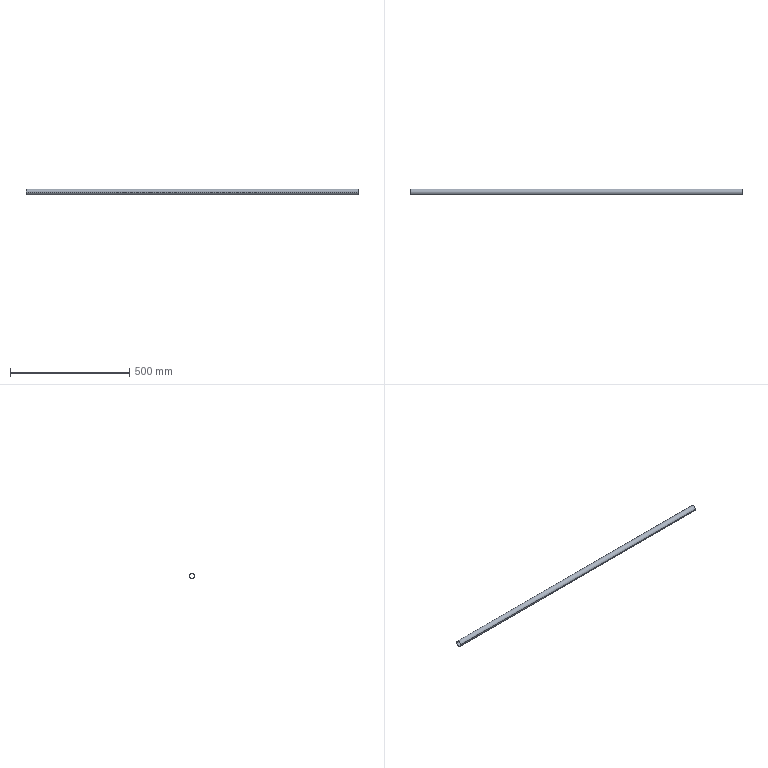Part | STEP file | 粉仓楼梯通道护栏栏杆2_Default<As Machined> | 1 solid | 6 faces | box 1390 x 25 x 25 mm | volume 153930 mm3 | cylinder 4 | plane 2 | commonest cylinder face diameters 22 x2 25 x2
STEP:
#1=CARTESIAN_POINT('',(0.,0.,0.));
#2=DIRECTION('',(0.,0.,1.));
#3=DIRECTION('',(1.,0.,0.));
#4=AXIS2_PLACEMENT_3D('',#1,#2,#3);
#5=CARTESIAN_POINT('',(695.,12.5,0.));
#6=VERTEX_POINT('',#5);
#7=CARTESIAN_POINT('',(695.,-12.5,0.));
#8=VERTEX_POINT('',#7);
#9=CARTESIAN_POINT('',(695.,0.,0.));
#10=DIRECTION('',(1.,0.,0.));
#11=DIRECTION('',(0.,1.,0.));
#12=AXIS2_PLACEMENT_3D('',#9,#10,#11);
#13=CIRCLE('',#12,12.5);
#14=CARTESIAN_POINT('',(695.,0.,0.));
#15=DIRECTION('',(-1.,0.,0.));
#16=DIRECTION('',(0.,-1.,0.));
#17=AXIS2_PLACEMENT_3D('',#14,#15,#16);
#18=CYLINDRICAL_SURFACE('',#17,12.5);
#19=CARTESIAN_POINT('',(3.142,0.));
#20=DIRECTION('',(-1.,0.));
#21=VECTOR('',#20,1.);
#22=LINE('',#19,#21);
#23=(GEOMETRIC_REPRESENTATION_CONTEXT(2)PARAMETRIC_REPRESENTATION_CONTEXT()REPRESENTATION_CONTEXT('',''));
#24=DEFINITIONAL_REPRESENTATION('',(#22),#23);
#25=PCURVE('',#18,#24);
#26=CARTESIAN_POINT('',(695.,0.,0.));
#27=DIRECTION('',(1.,0.,0.));
#28=DIRECTION('',(0.,1.,0.));
#29=AXIS2_PLACEMENT_3D('',#26,#27,#28);
#30=PLANE('',#29);
#31=CARTESIAN_POINT('',(0.,0.));
#32=DIRECTION('',(1.,0.));
#33=AXIS2_PLACEMENT_2D('',#31,#32);
#34=CIRCLE('',#33,12.5);
#35=(GEOMETRIC_REPRESENTATION_CONTEXT(2)PARAMETRIC_REPRESENTATION_CONTEXT()REPRESENTATION_CONTEXT('',''));
#36=DEFINITIONAL_REPRESENTATION('',(#34),#35);
#37=PCURVE('',#30,#36);
#38=SURFACE_CURVE('',#13,(#25,#37),.PCURVE_S1.);
#39=EDGE_CURVE('',#6,#8,#38,.T.);
#40=ORIENTED_EDGE('',*,*,#39,.F.);
#41=CARTESIAN_POINT('',(-695.,12.5,0.));
#42=VERTEX_POINT('',#41);
#43=CARTESIAN_POINT('',(695.,12.5,0.));
#44=DIRECTION('',(-1.,0.,0.));
#45=VECTOR('',#44,1.);
#46=LINE('',#43,#45);
#47=CARTESIAN_POINT('',(3.142,0.));
#48=DIRECTION('',(0.,1.));
#49=VECTOR('',#48,1.);
#50=LINE('',#47,#49);
#51=(GEOMETRIC_REPRESENTATION_CONTEXT(2)PARAMETRIC_REPRESENTATION_CONTEXT()REPRESENTATION_CONTEXT('',''));
#52=DEFINITIONAL_REPRESENTATION('',(#50),#51);
#53=PCURVE('',#18,#52);
#54=CARTESIAN_POINT('',(695.,0.,0.));
#55=DIRECTION('',(-1.,0.,0.));
#56=DIRECTION('',(0.,-1.,0.));
#57=AXIS2_PLACEMENT_3D('',#54,#55,#56);
#58=CYLINDRICAL_SURFACE('',#57,12.5);
#59=CARTESIAN_POINT('',(3.142,0.));
#60=DIRECTION('',(0.,1.));
#61=VECTOR('',#60,1.);
#62=LINE('',#59,#61);
#63=(GEOMETRIC_REPRESENTATION_CONTEXT(2)PARAMETRIC_REPRESENTATION_CONTEXT()REPRESENTATION_CONTEXT('',''));
#64=DEFINITIONAL_REPRESENTATION('',(#62),#63);
#65=PCURVE('',#58,#64);
#66=SURFACE_CURVE('',#46,(#53,#65),.PCURVE_S1.);
#67=EDGE_CURVE('',#6,#42,#66,.T.);
#68=ORIENTED_EDGE('',*,*,#67,.T.);
#69=CARTESIAN_POINT('',(-695.,-12.5,0.));
#70=VERTEX_POINT('',#69);
#71=CARTESIAN_POINT('',(-695.,0.,0.));
#72=DIRECTION('',(1.,0.,0.));
#73=DIRECTION('',(0.,1.,0.));
#74=AXIS2_PLACEMENT_3D('',#71,#72,#73);
#75=CIRCLE('',#74,12.5);
#76=CARTESIAN_POINT('',(3.142,1390.));
#77=DIRECTION('',(-1.,0.));
#78=VECTOR('',#77,1.);
#79=LINE('',#76,#78);
#80=(GEOMETRIC_REPRESENTATION_CONTEXT(2)PARAMETRIC_REPRESENTATION_CONTEXT()REPRESENTATION_CONTEXT('',''));
#81=DEFINITIONAL_REPRESENTATION('',(#79),#80);
#82=PCURVE('',#18,#81);
#83=CARTESIAN_POINT('',(-695.,0.,0.));
#84=DIRECTION('',(1.,0.,0.));
#85=DIRECTION('',(0.,1.,0.));
#86=AXIS2_PLACEMENT_3D('',#83,#84,#85);
#87=PLANE('',#86);
#88=CARTESIAN_POINT('',(0.,0.));
#89=DIRECTION('',(1.,0.));
#90=AXIS2_PLACEMENT_2D('',#88,#89);
#91=CIRCLE('',#90,12.5);
#92=(GEOMETRIC_REPRESENTATION_CONTEXT(2)PARAMETRIC_REPRESENTATION_CONTEXT()REPRESENTATION_CONTEXT('',''));
#93=DEFINITIONAL_REPRESENTATION('',(#91),#92);
#94=PCURVE('',#87,#93);
#95=SURFACE_CURVE('',#75,(#82,#94),.PCURVE_S1.);
#96=EDGE_CURVE('',#42,#70,#95,.T.);
#97=ORIENTED_EDGE('',*,*,#96,.T.);
#98=CARTESIAN_POINT('',(695.,-12.5,0.));
#99=DIRECTION('',(-1.,0.,0.));
#100=VECTOR('',#99,1.);
#101=LINE('',#98,#100);
#102=CARTESIAN_POINT('',(0.,0.));
#103=DIRECTION('',(0.,1.));
#104=VECTOR('',#103,1.);
#105=LINE('',#102,#104);
#106=(GEOMETRIC_REPRESENTATION_CONTEXT(2)PARAMETRIC_REPRESENTATION_CONTEXT()REPRESENTATION_CONTEXT('',''));
#107=DEFINITIONAL_REPRESENTATION('',(#105),#106);
#108=PCURVE('',#18,#107);
#109=CARTESIAN_POINT('',(6.283,0.));
#110=DIRECTION('',(0.,1.));
#111=VECTOR('',#110,1.);
#112=LINE('',#109,#111);
#113=(GEOMETRIC_REPRESENTATION_CONTEXT(2)PARAMETRIC_REPRESENTATION_CONTEXT()REPRESENTATION_CONTEXT('',''));
#114=DEFINITIONAL_REPRESENTATION('',(#112),#113);
#115=PCURVE('',#58,#114);
#116=SURFACE_CURVE('',#101,(#108,#115),.PCURVE_S1.);
#117=EDGE_CURVE('',#8,#70,#116,.T.);
#118=ORIENTED_EDGE('',*,*,#117,.F.);
#119=EDGE_LOOP('',(#40,#68,#97,#118));
#120=FACE_BOUND('',#119,.T.);
#121=ADVANCED_FACE('',(#120),#18,.T.);
#122=CARTESIAN_POINT('',(695.,-11.,0.));
#123=VERTEX_POINT('',#122);
#124=CARTESIAN_POINT('',(-695.,-11.,0.));
#125=VERTEX_POINT('',#124);
#126=CARTESIAN_POINT('',(695.,-11.,0.));
#127=DIRECTION('',(-1.,0.,0.));
#128=VECTOR('',#127,1.);
#129=LINE('',#126,#128);
#130=CARTESIAN_POINT('',(695.,0.,0.));
#131=DIRECTION('',(-1.,0.,0.));
#132=DIRECTION('',(0.,-1.,0.));
#133=AXIS2_PLACEMENT_3D('',#130,#131,#132);
#134=CYLINDRICAL_SURFACE('',#133,11.);
#135=CARTESIAN_POINT('',(6.283,0.));
#136=DIRECTION('',(0.,1.));
#137=VECTOR('',#136,1.);
#138=LINE('',#135,#137);
#139=(GEOMETRIC_REPRESENTATION_CONTEXT(2)PARAMETRIC_REPRESENTATION_CONTEXT()REPRESENTATION_CONTEXT('',''));
#140=DEFINITIONAL_REPRESENTATION('',(#138),#139);
#141=PCURVE('',#134,#140);
#142=CARTESIAN_POINT('',(695.,0.,0.));
#143=DIRECTION('',(-1.,0.,0.));
#144=DIRECTION('',(0.,-1.,0.));
#145=AXIS2_PLACEMENT_3D('',#142,#143,#144);
#146=CYLINDRICAL_SURFACE('',#145,11.);
#147=CARTESIAN_POINT('',(0.,0.));
#148=DIRECTION('',(0.,1.));
#149=VECTOR('',#148,1.);
#150=LINE('',#147,#149);
#151=(GEOMETRIC_REPRESENTATION_CONTEXT(2)PARAMETRIC_REPRESENTATION_CONTEXT()REPRESENTATION_CONTEXT('',''));
#152=DEFINITIONAL_REPRESENTATION('',(#150),#151);
#153=PCURVE('',#146,#152);
#154=SURFACE_CURVE('',#129,(#141,#153),.PCURVE_S1.);
#155=EDGE_CURVE('',#123,#125,#154,.T.);
#156=ORIENTED_EDGE('',*,*,#155,.T.);
#157=CARTESIAN_POINT('',(-695.,11.,0.));
#158=VERTEX_POINT('',#157);
#159=CARTESIAN_POINT('',(-695.,0.,0.));
#160=DIRECTION('',(1.,0.,0.));
#161=DIRECTION('',(0.,1.,0.));
#162=AXIS2_PLACEMENT_3D('',#159,#160,#161);
#163=CIRCLE('',#162,11.);
#164=CARTESIAN_POINT('',(9.425,1390.));
#165=DIRECTION('',(-1.,0.));
#166=VECTOR('',#165,1.);
#167=LINE('',#164,#166);
#168=(GEOMETRIC_REPRESENTATION_CONTEXT(2)PARAMETRIC_REPRESENTATION_CONTEXT()REPRESENTATION_CONTEXT('',''));
#169=DEFINITIONAL_REPRESENTATION('',(#167),#168);
#170=PCURVE('',#134,#169);
#171=CARTESIAN_POINT('',(0.,0.));
#172=DIRECTION('',(1.,0.));
#173=AXIS2_PLACEMENT_2D('',#171,#172);
#174=CIRCLE('',#173,11.);
#175=(GEOMETRIC_REPRESENTATION_CONTEXT(2)PARAMETRIC_REPRESENTATION_CONTEXT()REPRESENTATION_CONTEXT('',''));
#176=DEFINITIONAL_REPRESENTATION('',(#174),#175);
#177=PCURVE('',#87,#176);
#178=SURFACE_CURVE('',#163,(#170,#177),.PCURVE_S1.);
#179=EDGE_CURVE('',#125,#158,#178,.T.);
#180=ORIENTED_EDGE('',*,*,#179,.T.);
#181=CARTESIAN_POINT('',(695.,11.,0.));
#182=VERTEX_POINT('',#181);
#183=CARTESIAN_POINT('',(695.,11.,0.));
#184=DIRECTION('',(-1.,0.,0.));
#185=VECTOR('',#184,1.);
#186=LINE('',#183,#185);
#187=CARTESIAN_POINT('',(3.142,0.));
#188=DIRECTION('',(0.,1.));
#189=VECTOR('',#188,1.);
#190=LINE('',#187,#189);
#191=(GEOMETRIC_REPRESENTATION_CONTEXT(2)PARAMETRIC_REPRESENTATION_CONTEXT()REPRESENTATION_CONTEXT('',''));
#192=DEFINITIONAL_REPRESENTATION('',(#190),#191);
#193=PCURVE('',#134,#192);
#194=CARTESIAN_POINT('',(3.142,0.));
#195=DIRECTION('',(0.,1.));
#196=VECTOR('',#195,1.);
#197=LINE('',#194,#196);
#198=(GEOMETRIC_REPRESENTATION_CONTEXT(2)PARAMETRIC_REPRESENTATION_CONTEXT()REPRESENTATION_CONTEXT('',''));
#199=DEFINITIONAL_REPRESENTATION('',(#197),#198);
#200=PCURVE('',#146,#199);
#201=SURFACE_CURVE('',#186,(#193,#200),.PCURVE_S1.);
#202=EDGE_CURVE('',#182,#158,#201,.T.);
#203=ORIENTED_EDGE('',*,*,#202,.F.);
#204=CARTESIAN_POINT('',(695.,0.,0.));
#205=DIRECTION('',(1.,0.,0.));
#206=DIRECTION('',(0.,1.,0.));
#207=AXIS2_PLACEMENT_3D('',#204,#205,#206);
#208=CIRCLE('',#207,11.);
#209=CARTESIAN_POINT('',(9.425,0.));
#210=DIRECTION('',(-1.,0.));
#211=VECTOR('',#210,1.);
#212=LINE('',#209,#211);
#213=(GEOMETRIC_REPRESENTATION_CONTEXT(2)PARAMETRIC_REPRESENTATION_CONTEXT()REPRESENTATION_CONTEXT('',''));
#214=DEFINITIONAL_REPRESENTATION('',(#212),#213);
#215=PCURVE('',#134,#214);
#216=CARTESIAN_POINT('',(0.,0.));
#217=DIRECTION('',(1.,0.));
#218=AXIS2_PLACEMENT_2D('',#216,#217);
#219=CIRCLE('',#218,11.);
#220=(GEOMETRIC_REPRESENTATION_CONTEXT(2)PARAMETRIC_REPRESENTATION_CONTEXT()REPRESENTATION_CONTEXT('',''));
#221=DEFINITIONAL_REPRESENTATION('',(#219),#220);
#222=PCURVE('',#30,#221);
#223=SURFACE_CURVE('',#208,(#215,#222),.PCURVE_S1.);
#224=EDGE_CURVE('',#123,#182,#223,.T.);
#225=ORIENTED_EDGE('',*,*,#224,.F.);
#226=EDGE_LOOP('',(#156,#180,#203,#225));
#227=FACE_BOUND('',#226,.F.);
#228=ADVANCED_FACE('',(#227),#134,.F.);
#229=CARTESIAN_POINT('',(-695.,0.,0.));
#230=DIRECTION('',(1.,0.,0.));
#231=DIRECTION('',(0.,1.,0.));
#232=AXIS2_PLACEMENT_3D('',#229,#230,#231);
#233=CIRCLE('',#232,11.);
#234=CARTESIAN_POINT('',(3.142,1390.));
#235=DIRECTION('',(-1.,0.));
#236=VECTOR('',#235,1.);
#237=LINE('',#234,#236);
#238=(GEOMETRIC_REPRESENTATION_CONTEXT(2)PARAMETRIC_REPRESENTATION_CONTEXT()REPRESENTATION_CONTEXT('',''));
#239=DEFINITIONAL_REPRESENTATION('',(#237),#238);
#240=PCURVE('',#146,#239);
#241=CARTESIAN_POINT('',(0.,0.));
#242=DIRECTION('',(1.,0.));
#243=AXIS2_PLACEMENT_2D('',#241,#242);
#244=CIRCLE('',#243,11.);
#245=(GEOMETRIC_REPRESENTATION_CONTEXT(2)PARAMETRIC_REPRESENTATION_CONTEXT()REPRESENTATION_CONTEXT('',''));
#246=DEFINITIONAL_REPRESENTATION('',(#244),#245);
#247=PCURVE('',#87,#246);
#248=SURFACE_CURVE('',#233,(#240,#247),.PCURVE_S1.);
#249=EDGE_CURVE('',#158,#125,#248,.T.);
#250=ORIENTED_EDGE('',*,*,#249,.T.);
#251=ORIENTED_EDGE('',*,*,#155,.F.);
#252=CARTESIAN_POINT('',(695.,0.,0.));
#253=DIRECTION('',(1.,0.,0.));
#254=DIRECTION('',(0.,1.,0.));
#255=AXIS2_PLACEMENT_3D('',#252,#253,#254);
#256=CIRCLE('',#255,11.);
#257=CARTESIAN_POINT('',(3.142,0.));
#258=DIRECTION('',(-1.,0.));
#259=VECTOR('',#258,1.);
#260=LINE('',#257,#259);
#261=(GEOMETRIC_REPRESENTATION_CONTEXT(2)PARAMETRIC_REPRESENTATION_CONTEXT()REPRESENTATION_CONTEXT('',''));
#262=DEFINITIONAL_REPRESENTATION('',(#260),#261);
#263=PCURVE('',#146,#262);
#264=CARTESIAN_POINT('',(0.,0.));
#265=DIRECTION('',(1.,0.));
#266=AXIS2_PLACEMENT_2D('',#264,#265);
#267=CIRCLE('',#266,11.);
#268=(GEOMETRIC_REPRESENTATION_CONTEXT(2)PARAMETRIC_REPRESENTATION_CONTEXT()REPRESENTATION_CONTEXT('',''));
#269=DEFINITIONAL_REPRESENTATION('',(#267),#268);
#270=PCURVE('',#30,#269);
#271=SURFACE_CURVE('',#256,(#263,#270),.PCURVE_S1.);
#272=EDGE_CURVE('',#182,#123,#271,.T.);
#273=ORIENTED_EDGE('',*,*,#272,.F.);
#274=ORIENTED_EDGE('',*,*,#202,.T.);
#275=EDGE_LOOP('',(#250,#251,#273,#274));
#276=FACE_BOUND('',#275,.F.);
#277=ADVANCED_FACE('',(#276),#146,.F.);
#278=ORIENTED_EDGE('',*,*,#67,.F.);
#279=CARTESIAN_POINT('',(695.,0.,0.));
#280=DIRECTION('',(1.,0.,0.));
#281=DIRECTION('',(0.,1.,0.));
#282=AXIS2_PLACEMENT_3D('',#279,#280,#281);
#283=CIRCLE('',#282,12.5);
#284=CARTESIAN_POINT('',(9.425,0.));
#285=DIRECTION('',(-1.,0.));
#286=VECTOR('',#285,1.);
#287=LINE('',#284,#286);
#288=(GEOMETRIC_REPRESENTATION_CONTEXT(2)PARAMETRIC_REPRESENTATION_CONTEXT()REPRESENTATION_CONTEXT('',''));
#289=DEFINITIONAL_REPRESENTATION('',(#287),#288);
#290=PCURVE('',#58,#289);
#291=CARTESIAN_POINT('',(0.,0.));
#292=DIRECTION('',(1.,0.));
#293=AXIS2_PLACEMENT_2D('',#291,#292);
#294=CIRCLE('',#293,12.5);
#295=(GEOMETRIC_REPRESENTATION_CONTEXT(2)PARAMETRIC_REPRESENTATION_CONTEXT()REPRESENTATION_CONTEXT('',''));
#296=DEFINITIONAL_REPRESENTATION('',(#294),#295);
#297=PCURVE('',#30,#296);
#298=SURFACE_CURVE('',#283,(#290,#297),.PCURVE_S1.);
#299=EDGE_CURVE('',#8,#6,#298,.T.);
#300=ORIENTED_EDGE('',*,*,#299,.F.);
#301=ORIENTED_EDGE('',*,*,#117,.T.);
#302=CARTESIAN_POINT('',(-695.,0.,0.));
#303=DIRECTION('',(1.,0.,0.));
#304=DIRECTION('',(0.,1.,0.));
#305=AXIS2_PLACEMENT_3D('',#302,#303,#304);
#306=CIRCLE('',#305,12.5);
#307=CARTESIAN_POINT('',(9.425,1390.));
#308=DIRECTION('',(-1.,0.));
#309=VECTOR('',#308,1.);
#310=LINE('',#307,#309);
#311=(GEOMETRIC_REPRESENTATION_CONTEXT(2)PARAMETRIC_REPRESENTATION_CONTEXT()REPRESENTATION_CONTEXT('',''));
#312=DEFINITIONAL_REPRESENTATION('',(#310),#311);
#313=PCURVE('',#58,#312);
#314=CARTESIAN_POINT('',(0.,0.));
#315=DIRECTION('',(1.,0.));
#316=AXIS2_PLACEMENT_2D('',#314,#315);
#317=CIRCLE('',#316,12.5);
#318=(GEOMETRIC_REPRESENTATION_CONTEXT(2)PARAMETRIC_REPRESENTATION_CONTEXT()REPRESENTATION_CONTEXT('',''));
#319=DEFINITIONAL_REPRESENTATION('',(#317),#318);
#320=PCURVE('',#87,#319);
#321=SURFACE_CURVE('',#306,(#313,#320),.PCURVE_S1.);
#322=EDGE_CURVE('',#70,#42,#321,.T.);
#323=ORIENTED_EDGE('',*,*,#322,.T.);
#324=EDGE_LOOP('',(#278,#300,#301,#323));
#325=FACE_BOUND('',#324,.T.);
#326=ADVANCED_FACE('',(#325),#58,.T.);
#327=ORIENTED_EDGE('',*,*,#224,.F.);
#328=ORIENTED_EDGE('',*,*,#272,.F.);
#329=EDGE_LOOP('',(#327,#328));
#330=FACE_BOUND('',#329,.T.);
#331=ORIENTED_EDGE('',*,*,#299,.T.);
#332=ORIENTED_EDGE('',*,*,#39,.T.);
#333=EDGE_LOOP('',(#331,#332));
#334=FACE_BOUND('',#333,.T.);
#335=ADVANCED_FACE('',(#330,#334),#30,.T.);
#336=ORIENTED_EDGE('',*,*,#179,.T.);
#337=ORIENTED_EDGE('',*,*,#249,.T.);
#338=EDGE_LOOP('',(#336,#337));
#339=FACE_BOUND('',#338,.T.);
#340=ORIENTED_EDGE('',*,*,#322,.F.);
#341=ORIENTED_EDGE('',*,*,#96,.F.);
#342=EDGE_LOOP('',(#340,#341));
#343=FACE_BOUND('',#342,.T.);
#344=ADVANCED_FACE('',(#339,#343),#87,.F.);
#345=CLOSED_SHELL('',(#121,#228,#277,#326,#335,#344));
#346=MANIFOLD_SOLID_BREP('',#345);
#347=(LENGTH_UNIT()NAMED_UNIT(*)SI_UNIT(.MILLI.,.METRE.));
#348=UNCERTAINTY_MEASURE_WITH_UNIT(LENGTH_MEASURE(0.0000001),#347,'','');
#349=(NAMED_UNIT(*)PLANE_ANGLE_UNIT()SI_UNIT($,.RADIAN.));
#350=(NAMED_UNIT(*)SI_UNIT($,.STERADIAN.)SOLID_ANGLE_UNIT());
#351=(GEOMETRIC_REPRESENTATION_CONTEXT(3)GLOBAL_UNCERTAINTY_ASSIGNED_CONTEXT((#348))GLOBAL_UNIT_ASSIGNED_CONTEXT((#347,#349,#350))REPRESENTATION_CONTEXT('',''));
#352=ADVANCED_BREP_SHAPE_REPRESENTATION('',(#4,#346),#351);